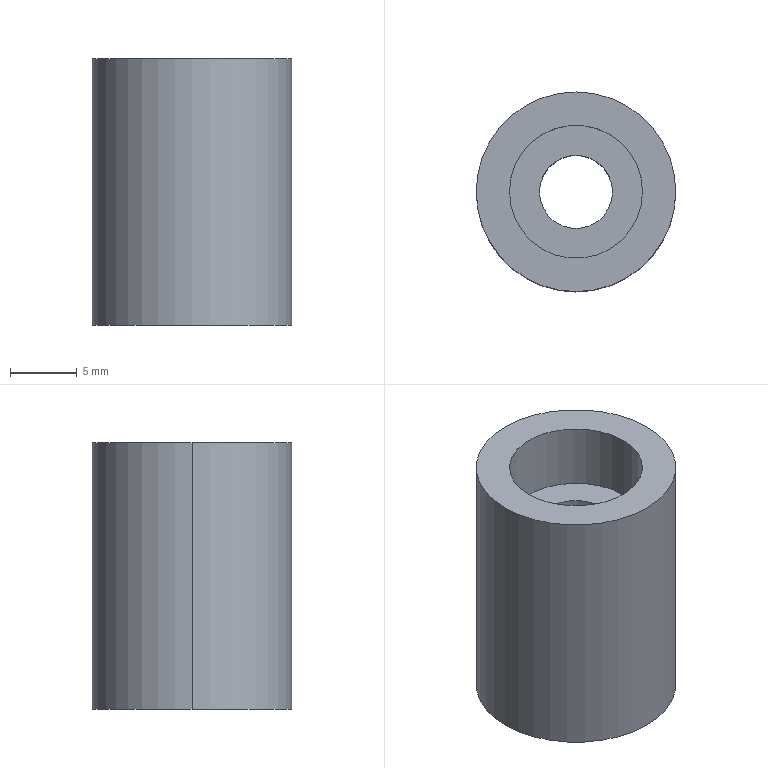Part | NX | features BREP 1 | 1 solid | 9 faces | box 15 x 15 x 20 mm | volume 2785 mm3 | cylinder 6 | plane 3 | commonest cylinder face diameters 5.5 x2 10 x2 15 x2
STEP:
#1=CARTESIAN_POINT('',(-5.,0.,20.));
#2=VERTEX_POINT('',#1);
#3=CARTESIAN_POINT('',(-5.,0.,15.));
#4=VERTEX_POINT('',#3);
#5=CARTESIAN_POINT('',(-5.,0.,20.));
#6=DIRECTION('',(0.,0.,1.));
#7=VECTOR('',#6,1000.);
#8=LINE('',#5,#7);
#9=EDGE_CURVE('',#2,#4,#8,.F.);
#10=ORIENTED_EDGE('',*,*,#9,.T.);
#11=CARTESIAN_POINT('',(5.,0.,15.));
#12=VERTEX_POINT('',#11);
#13=CARTESIAN_POINT('',(0.,0.,15.));
#14=DIRECTION('',(0.,0.,1.));
#15=DIRECTION('',(1.,0.,0.));
#16=AXIS2_PLACEMENT_3D('',#13,#14,#15);
#17=CIRCLE('',#16,5.);
#18=EDGE_CURVE('',#12,#4,#17,.T.);
#19=ORIENTED_EDGE('',*,*,#18,.F.);
#20=CARTESIAN_POINT('',(5.,0.,20.));
#21=VERTEX_POINT('',#20);
#22=CARTESIAN_POINT('',(5.,0.,20.));
#23=DIRECTION('',(0.,0.,1.));
#24=VECTOR('',#23,1000.);
#25=LINE('',#22,#24);
#26=EDGE_CURVE('',#21,#12,#25,.F.);
#27=ORIENTED_EDGE('',*,*,#26,.F.);
#28=CARTESIAN_POINT('',(0.,0.,20.));
#29=DIRECTION('',(0.,0.,1.));
#30=DIRECTION('',(1.,0.,0.));
#31=AXIS2_PLACEMENT_3D('',#28,#29,#30);
#32=CIRCLE('',#31,5.);
#33=EDGE_CURVE('',#21,#2,#32,.T.);
#34=ORIENTED_EDGE('',*,*,#33,.T.);
#35=EDGE_LOOP('',(#10,#19,#27,#34));
#36=FACE_BOUND('',#35,.T.);
#37=CARTESIAN_POINT('',(0.,0.,20.));
#38=DIRECTION('',(0.,0.,1.));
#39=DIRECTION('',(1.,0.,0.));
#40=AXIS2_PLACEMENT_3D('',#37,#38,#39);
#41=CYLINDRICAL_SURFACE('',#40,5.);
#42=ADVANCED_FACE('',(#36),#41,.F.);
#43=ORIENTED_EDGE('',*,*,#18,.T.);
#44=CARTESIAN_POINT('',(0.,0.,15.));
#45=DIRECTION('',(0.,0.,1.));
#46=DIRECTION('',(1.,0.,0.));
#47=AXIS2_PLACEMENT_3D('',#44,#45,#46);
#48=CIRCLE('',#47,5.);
#49=EDGE_CURVE('',#4,#12,#48,.T.);
#50=ORIENTED_EDGE('',*,*,#49,.T.);
#51=EDGE_LOOP('',(#43,#50));
#52=FACE_BOUND('',#51,.T.);
#53=CARTESIAN_POINT('',(2.75,0.,15.));
#54=VERTEX_POINT('',#53);
#55=CARTESIAN_POINT('',(-2.75,0.,15.));
#56=VERTEX_POINT('',#55);
#57=CARTESIAN_POINT('',(0.,0.,15.));
#58=DIRECTION('',(0.,0.,1.));
#59=DIRECTION('',(1.,0.,0.));
#60=AXIS2_PLACEMENT_3D('',#57,#58,#59);
#61=CIRCLE('',#60,2.75);
#62=EDGE_CURVE('',#54,#56,#61,.T.);
#63=ORIENTED_EDGE('',*,*,#62,.F.);
#64=CARTESIAN_POINT('',(0.,0.,15.));
#65=DIRECTION('',(0.,0.,1.));
#66=DIRECTION('',(1.,0.,0.));
#67=AXIS2_PLACEMENT_3D('',#64,#65,#66);
#68=CIRCLE('',#67,2.75);
#69=EDGE_CURVE('',#56,#54,#68,.T.);
#70=ORIENTED_EDGE('',*,*,#69,.F.);
#71=EDGE_LOOP('',(#63,#70));
#72=FACE_BOUND('',#71,.T.);
#73=CARTESIAN_POINT('',(2.75,0.,15.));
#74=DIRECTION('',(0.,0.,-1.));
#75=DIRECTION('',(-1.,0.,0.));
#76=AXIS2_PLACEMENT_3D('',#73,#74,#75);
#77=PLANE('',#76);
#78=ADVANCED_FACE('',(#52,#72),#77,.F.);
#79=CARTESIAN_POINT('',(-2.75,0.,0.));
#80=VERTEX_POINT('',#79);
#81=CARTESIAN_POINT('',(-2.75,0.,20.));
#82=DIRECTION('',(0.,0.,1.));
#83=VECTOR('',#82,1000.);
#84=LINE('',#81,#83);
#85=EDGE_CURVE('',#56,#80,#84,.F.);
#86=ORIENTED_EDGE('',*,*,#85,.T.);
#87=CARTESIAN_POINT('',(2.75,0.,0.));
#88=VERTEX_POINT('',#87);
#89=CARTESIAN_POINT('',(0.,0.,0.));
#90=DIRECTION('',(0.,0.,1.));
#91=DIRECTION('',(1.,0.,0.));
#92=AXIS2_PLACEMENT_3D('',#89,#90,#91);
#93=CIRCLE('',#92,2.75);
#94=EDGE_CURVE('',#88,#80,#93,.T.);
#95=ORIENTED_EDGE('',*,*,#94,.F.);
#96=CARTESIAN_POINT('',(2.75,0.,20.));
#97=DIRECTION('',(0.,0.,1.));
#98=VECTOR('',#97,1000.);
#99=LINE('',#96,#98);
#100=EDGE_CURVE('',#54,#88,#99,.F.);
#101=ORIENTED_EDGE('',*,*,#100,.F.);
#102=ORIENTED_EDGE('',*,*,#62,.T.);
#103=EDGE_LOOP('',(#86,#95,#101,#102));
#104=FACE_BOUND('',#103,.T.);
#105=CARTESIAN_POINT('',(0.,0.,20.));
#106=DIRECTION('',(0.,0.,1.));
#107=DIRECTION('',(1.,0.,0.));
#108=AXIS2_PLACEMENT_3D('',#105,#106,#107);
#109=CYLINDRICAL_SURFACE('',#108,2.75);
#110=ADVANCED_FACE('',(#104),#109,.F.);
#111=CARTESIAN_POINT('',(-7.5,0.,0.));
#112=VERTEX_POINT('',#111);
#113=CARTESIAN_POINT('',(7.5,0.,0.));
#114=VERTEX_POINT('',#113);
#115=CARTESIAN_POINT('',(0.,0.,0.));
#116=DIRECTION('',(0.,0.,1.));
#117=DIRECTION('',(1.,0.,0.));
#118=AXIS2_PLACEMENT_3D('',#115,#116,#117);
#119=CIRCLE('',#118,7.5);
#120=EDGE_CURVE('',#112,#114,#119,.T.);
#121=ORIENTED_EDGE('',*,*,#120,.F.);
#122=CARTESIAN_POINT('',(0.,0.,0.));
#123=DIRECTION('',(0.,0.,1.));
#124=DIRECTION('',(1.,0.,0.));
#125=AXIS2_PLACEMENT_3D('',#122,#123,#124);
#126=CIRCLE('',#125,7.5);
#127=EDGE_CURVE('',#114,#112,#126,.T.);
#128=ORIENTED_EDGE('',*,*,#127,.F.);
#129=EDGE_LOOP('',(#121,#128));
#130=FACE_BOUND('',#129,.T.);
#131=ORIENTED_EDGE('',*,*,#94,.T.);
#132=CARTESIAN_POINT('',(0.,0.,0.));
#133=DIRECTION('',(0.,0.,1.));
#134=DIRECTION('',(1.,0.,0.));
#135=AXIS2_PLACEMENT_3D('',#132,#133,#134);
#136=CIRCLE('',#135,2.75);
#137=EDGE_CURVE('',#80,#88,#136,.T.);
#138=ORIENTED_EDGE('',*,*,#137,.T.);
#139=EDGE_LOOP('',(#131,#138));
#140=FACE_BOUND('',#139,.T.);
#141=CARTESIAN_POINT('',(0.,0.,0.));
#142=DIRECTION('',(0.,0.,1.));
#143=DIRECTION('',(1.,0.,0.));
#144=AXIS2_PLACEMENT_3D('',#141,#142,#143);
#145=PLANE('',#144);
#146=ADVANCED_FACE('',(#130,#140),#145,.F.);
#147=CARTESIAN_POINT('',(-7.5,0.,20.));
#148=VERTEX_POINT('',#147);
#149=CARTESIAN_POINT('',(7.5,0.,20.));
#150=VERTEX_POINT('',#149);
#151=CARTESIAN_POINT('',(0.,0.,20.));
#152=DIRECTION('',(0.,0.,1.));
#153=DIRECTION('',(1.,0.,0.));
#154=AXIS2_PLACEMENT_3D('',#151,#152,#153);
#155=CIRCLE('',#154,7.5);
#156=EDGE_CURVE('',#148,#150,#155,.T.);
#157=ORIENTED_EDGE('',*,*,#156,.T.);
#158=CARTESIAN_POINT('',(0.,0.,20.));
#159=DIRECTION('',(0.,0.,1.));
#160=DIRECTION('',(1.,0.,0.));
#161=AXIS2_PLACEMENT_3D('',#158,#159,#160);
#162=CIRCLE('',#161,7.5);
#163=EDGE_CURVE('',#150,#148,#162,.T.);
#164=ORIENTED_EDGE('',*,*,#163,.T.);
#165=EDGE_LOOP('',(#157,#164));
#166=FACE_BOUND('',#165,.T.);
#167=ORIENTED_EDGE('',*,*,#33,.F.);
#168=CARTESIAN_POINT('',(0.,0.,20.));
#169=DIRECTION('',(0.,0.,1.));
#170=DIRECTION('',(1.,0.,0.));
#171=AXIS2_PLACEMENT_3D('',#168,#169,#170);
#172=CIRCLE('',#171,5.);
#173=EDGE_CURVE('',#2,#21,#172,.T.);
#174=ORIENTED_EDGE('',*,*,#173,.F.);
#175=EDGE_LOOP('',(#167,#174));
#176=FACE_BOUND('',#175,.T.);
#177=CARTESIAN_POINT('',(0.,0.,20.));
#178=DIRECTION('',(0.,0.,1.));
#179=DIRECTION('',(1.,0.,0.));
#180=AXIS2_PLACEMENT_3D('',#177,#178,#179);
#181=PLANE('',#180);
#182=ADVANCED_FACE('',(#166,#176),#181,.T.);
#183=CARTESIAN_POINT('',(7.5,0.,20.));
#184=DIRECTION('',(0.,0.,-1.));
#185=VECTOR('',#184,1000.);
#186=LINE('',#183,#185);
#187=EDGE_CURVE('',#150,#114,#186,.T.);
#188=ORIENTED_EDGE('',*,*,#187,.F.);
#189=ORIENTED_EDGE('',*,*,#156,.F.);
#190=CARTESIAN_POINT('',(-7.5,0.,20.));
#191=DIRECTION('',(0.,0.,-1.));
#192=VECTOR('',#191,1000.);
#193=LINE('',#190,#192);
#194=EDGE_CURVE('',#148,#112,#193,.T.);
#195=ORIENTED_EDGE('',*,*,#194,.T.);
#196=ORIENTED_EDGE('',*,*,#120,.T.);
#197=EDGE_LOOP('',(#188,#189,#195,#196));
#198=FACE_BOUND('',#197,.T.);
#199=CARTESIAN_POINT('',(0.,0.,20.));
#200=DIRECTION('',(0.,0.,-1.));
#201=DIRECTION('',(-1.,0.,0.));
#202=AXIS2_PLACEMENT_3D('',#199,#200,#201);
#203=CYLINDRICAL_SURFACE('',#202,7.5);
#204=ADVANCED_FACE('',(#198),#203,.T.);
#205=ORIENTED_EDGE('',*,*,#163,.F.);
#206=ORIENTED_EDGE('',*,*,#187,.T.);
#207=ORIENTED_EDGE('',*,*,#127,.T.);
#208=ORIENTED_EDGE('',*,*,#194,.F.);
#209=EDGE_LOOP('',(#205,#206,#207,#208));
#210=FACE_BOUND('',#209,.T.);
#211=CARTESIAN_POINT('',(0.,0.,20.));
#212=DIRECTION('',(0.,0.,-1.));
#213=DIRECTION('',(-1.,0.,0.));
#214=AXIS2_PLACEMENT_3D('',#211,#212,#213);
#215=CYLINDRICAL_SURFACE('',#214,7.5);
#216=ADVANCED_FACE('',(#210),#215,.T.);
#217=ORIENTED_EDGE('',*,*,#137,.F.);
#218=ORIENTED_EDGE('',*,*,#85,.F.);
#219=ORIENTED_EDGE('',*,*,#69,.T.);
#220=ORIENTED_EDGE('',*,*,#100,.T.);
#221=EDGE_LOOP('',(#217,#218,#219,#220));
#222=FACE_BOUND('',#221,.T.);
#223=CARTESIAN_POINT('',(0.,0.,20.));
#224=DIRECTION('',(0.,0.,1.));
#225=DIRECTION('',(1.,0.,0.));
#226=AXIS2_PLACEMENT_3D('',#223,#224,#225);
#227=CYLINDRICAL_SURFACE('',#226,2.75);
#228=ADVANCED_FACE('',(#222),#227,.F.);
#229=ORIENTED_EDGE('',*,*,#49,.F.);
#230=ORIENTED_EDGE('',*,*,#9,.F.);
#231=ORIENTED_EDGE('',*,*,#173,.T.);
#232=ORIENTED_EDGE('',*,*,#26,.T.);
#233=EDGE_LOOP('',(#229,#230,#231,#232));
#234=FACE_BOUND('',#233,.T.);
#235=CARTESIAN_POINT('',(0.,0.,20.));
#236=DIRECTION('',(0.,0.,1.));
#237=DIRECTION('',(1.,0.,0.));
#238=AXIS2_PLACEMENT_3D('',#235,#236,#237);
#239=CYLINDRICAL_SURFACE('',#238,5.);
#240=ADVANCED_FACE('',(#234),#239,.F.);
#241=CLOSED_SHELL('',(#42,#78,#110,#146,#182,#204,#216,#228,#240));
#242=MANIFOLD_SOLID_BREP('',#241);
#243=(LENGTH_UNIT()NAMED_UNIT(*)SI_UNIT(.MILLI.,.METRE.));
#244=UNCERTAINTY_MEASURE_WITH_UNIT(LENGTH_MEASURE(0.00001),#243,'','');
#245=(NAMED_UNIT(*)PLANE_ANGLE_UNIT()SI_UNIT($,.RADIAN.));
#246=(NAMED_UNIT(*)SI_UNIT($,.STERADIAN.)SOLID_ANGLE_UNIT());
#247=(GEOMETRIC_REPRESENTATION_CONTEXT(3)GLOBAL_UNCERTAINTY_ASSIGNED_CONTEXT((#244))GLOBAL_UNIT_ASSIGNED_CONTEXT((#243,#245,#246))REPRESENTATION_CONTEXT('',''));
#248=ADVANCED_BREP_SHAPE_REPRESENTATION('',(#242),#247);